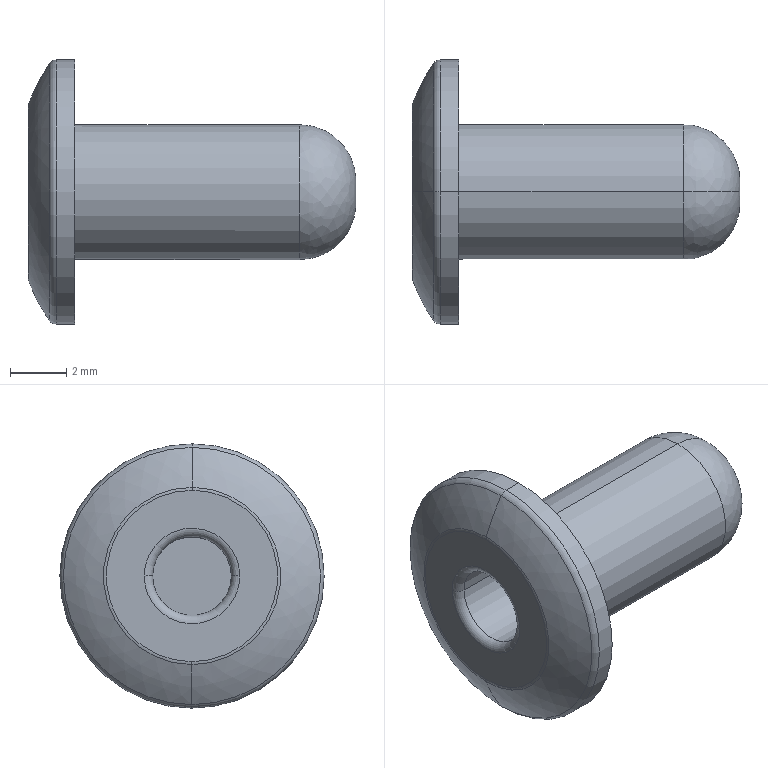Part | SolidWorks | features BaseBody 1 | 1 solid | 22 faces | box 11.653 x 9.4 x 9.401 mm | volume 238.079 mm3 | torus 8 | cylinder 6 | spline 4 | plane 4 | commonest cylinder face diameters 2.8 x2 4.8 x2 9.4 x2
STEP:
#1=CARTESIAN_POINT('',(-249.559,-95.819,-153.081));
#2=VERTEX_POINT('',#1);
#3=CARTESIAN_POINT('',(-249.804,-95.819,-153.208));
#4=VERTEX_POINT('',#3);
#5=CARTESIAN_POINT('',(-249.559,-95.819,-153.381));
#6=DIRECTION('',(0.00003827,-1.,-0.0004455));
#7=DIRECTION('',(0.0008339,-0.0004454,1.));
#8=AXIS2_PLACEMENT_3D('',#5,#6,#7);
#9=CIRCLE('',#8,0.3);
#10=EDGE_CURVE('',#2,#4,#9,.T.);
#11=ORIENTED_EDGE('',*,*,#10,.T.);
#12=CARTESIAN_POINT('',(-249.812,-95.815,-162.354));
#13=VERTEX_POINT('',#12);
#14=CARTESIAN_POINT('',(-249.808,-95.817,-157.781));
#15=DIRECTION('',(1.,0.00003864,-0.0008339));
#16=DIRECTION('',(0.0008339,-0.0004544,1.));
#17=AXIS2_PLACEMENT_3D('',#14,#15,#16);
#18=CIRCLE('',#17,4.573);
#19=EDGE_CURVE('',#4,#13,#18,.T.);
#20=ORIENTED_EDGE('',*,*,#19,.T.);
#21=CARTESIAN_POINT('',(-249.566,-95.815,-162.481));
#22=VERTEX_POINT('',#21);
#23=CARTESIAN_POINT('',(-249.566,-95.815,-162.181));
#24=DIRECTION('',(-0.00003827,1.,0.0004455));
#25=DIRECTION('',(-0.0008339,0.0004454,-1.));
#26=AXIS2_PLACEMENT_3D('',#23,#24,#25);
#27=CIRCLE('',#26,0.3);
#28=EDGE_CURVE('',#22,#13,#27,.T.);
#29=ORIENTED_EDGE('',*,*,#28,.F.);
#30=CARTESIAN_POINT('',(-249.562,-95.817,-157.781));
#31=DIRECTION('',(1.,0.00003864,-0.0008339));
#32=DIRECTION('',(0.0008339,-0.0004454,1.));
#33=AXIS2_PLACEMENT_3D('',#30,#31,#32);
#34=CIRCLE('',#33,4.7);
#35=EDGE_CURVE('',#2,#22,#34,.T.);
#36=ORIENTED_EDGE('',*,*,#35,.F.);
#37=EDGE_LOOP('',(#11,#20,#29,#36));
#38=FACE_OUTER_BOUND('',#37,.T.);
#39=CARTESIAN_POINT('',(-249.562,-95.817,-157.781));
#40=DIRECTION('',(1.,0.00003864,-0.0008339));
#41=DIRECTION('',(0.0008337,0.005616,1.));
#42=AXIS2_PLACEMENT_3D('',#39,#40,#41);
#43=TOROIDAL_SURFACE('',#42,4.4,0.3);
#44=ADVANCED_FACE('',(#38),#43,.T.);
#45=CARTESIAN_POINT('',(-248.919,-95.815,-162.481));
#46=VERTEX_POINT('',#45);
#47=CARTESIAN_POINT('',(-248.912,-95.819,-153.081));
#48=VERTEX_POINT('',#47);
#49=CARTESIAN_POINT('',(-248.916,-95.817,-157.781));
#50=DIRECTION('',(-1.,-0.00003864,0.0008339));
#51=DIRECTION('',(-0.0008339,0.0004454,-1.));
#52=AXIS2_PLACEMENT_3D('',#49,#50,#51);
#53=CIRCLE('',#52,4.7);
#54=EDGE_CURVE('',#46,#48,#53,.T.);
#55=ORIENTED_EDGE('',*,*,#54,.T.);
#56=CARTESIAN_POINT('',(-249.559,-95.819,-153.081));
#57=DIRECTION('',(1.,0.00003864,-0.0008339));
#58=VECTOR('',#57,1000.);
#59=LINE('',#56,#58);
#60=EDGE_CURVE('',#2,#48,#59,.T.);
#61=ORIENTED_EDGE('',*,*,#60,.F.);
#62=ORIENTED_EDGE('',*,*,#35,.T.);
#63=CARTESIAN_POINT('',(-249.566,-95.815,-162.481));
#64=DIRECTION('',(1.,0.00003864,-0.0008339));
#65=VECTOR('',#64,1000.);
#66=LINE('',#63,#65);
#67=EDGE_CURVE('',#22,#46,#66,.T.);
#68=ORIENTED_EDGE('',*,*,#67,.T.);
#69=EDGE_LOOP('',(#55,#61,#62,#68));
#70=FACE_OUTER_BOUND('',#69,.T.);
#71=CARTESIAN_POINT('',(-250.566,-95.817,-157.78));
#72=DIRECTION('',(1.,0.00003864,-0.0008339));
#73=DIRECTION('',(0.0008339,-0.0004454,1.));
#74=AXIS2_PLACEMENT_3D('',#71,#72,#73);
#75=CYLINDRICAL_SURFACE('',#74,4.7);
#76=ADVANCED_FACE('',(#70),#75,.T.);
#77=CARTESIAN_POINT('',(-248.916,-95.817,-157.781));
#78=DIRECTION('',(-1.,-0.00003864,0.0008339));
#79=DIRECTION('',(0.0008339,-0.0004454,1.));
#80=AXIS2_PLACEMENT_3D('',#77,#78,#79);
#81=CIRCLE('',#80,4.7);
#82=EDGE_CURVE('',#48,#46,#81,.T.);
#83=ORIENTED_EDGE('',*,*,#82,.T.);
#84=ORIENTED_EDGE('',*,*,#67,.F.);
#85=CARTESIAN_POINT('',(-249.562,-95.817,-157.781));
#86=DIRECTION('',(1.,0.00003864,-0.0008339));
#87=DIRECTION('',(-0.0008339,0.0004454,-1.));
#88=AXIS2_PLACEMENT_3D('',#85,#86,#87);
#89=CIRCLE('',#88,4.7);
#90=EDGE_CURVE('',#22,#2,#89,.T.);
#91=ORIENTED_EDGE('',*,*,#90,.T.);
#92=ORIENTED_EDGE('',*,*,#60,.T.);
#93=EDGE_LOOP('',(#83,#84,#91,#92));
#94=FACE_OUTER_BOUND('',#93,.T.);
#95=CARTESIAN_POINT('',(-250.566,-95.817,-157.78));
#96=DIRECTION('',(1.,0.00003864,-0.0008339));
#97=DIRECTION('',(0.0008339,-0.0004454,1.));
#98=AXIS2_PLACEMENT_3D('',#95,#96,#97);
#99=CYLINDRICAL_SURFACE('',#98,4.7);
#100=ADVANCED_FACE('',(#94),#99,.T.);
#101=ORIENTED_EDGE('',*,*,#28,.T.);
#102=CARTESIAN_POINT('',(-249.808,-95.817,-157.781));
#103=DIRECTION('',(1.,0.00003864,-0.0008339));
#104=DIRECTION('',(-0.0008339,0.0004544,-1.));
#105=AXIS2_PLACEMENT_3D('',#102,#103,#104);
#106=CIRCLE('',#105,4.573);
#107=EDGE_CURVE('',#13,#4,#106,.T.);
#108=ORIENTED_EDGE('',*,*,#107,.T.);
#109=ORIENTED_EDGE('',*,*,#10,.F.);
#110=ORIENTED_EDGE('',*,*,#90,.F.);
#111=EDGE_LOOP('',(#101,#108,#109,#110));
#112=FACE_OUTER_BOUND('',#111,.T.);
#113=CARTESIAN_POINT('',(-249.562,-95.817,-157.781));
#114=DIRECTION('',(1.,0.00003864,-0.0008339));
#115=DIRECTION('',(-0.0008337,-0.005616,-1.));
#116=AXIS2_PLACEMENT_3D('',#113,#114,#115);
#117=TOROIDAL_SURFACE('',#116,4.4,0.3);
#118=ADVANCED_FACE('',(#112),#117,.T.);
#119=CARTESIAN_POINT('',(-250.545,-95.819,-154.63));
#120=VERTEX_POINT('',#119);
#121=CARTESIAN_POINT('',(-249.804,-95.819,-153.208));
#122=CARTESIAN_POINT('',(-249.907,-95.819,-153.354));
#123=CARTESIAN_POINT('',(-250.1,-95.819,-153.655));
#124=CARTESIAN_POINT('',(-250.348,-95.819,-154.131));
#125=CARTESIAN_POINT('',(-250.484,-95.819,-154.462));
#126=CARTESIAN_POINT('',(-250.545,-95.819,-154.63));
#127=B_SPLINE_CURVE_WITH_KNOTS('',3,(#121,#122,#123,#124,#125,#126),.UNSPECIFIED.,.F.,.F.,(4,1,1,4),(0.,0.3333,0.6667,1.),.UNSPECIFIED.);
#128=EDGE_CURVE('',#4,#120,#127,.T.);
#129=ORIENTED_EDGE('',*,*,#128,.F.);
#130=ORIENTED_EDGE('',*,*,#107,.F.);
#131=CARTESIAN_POINT('',(-250.55,-95.816,-160.93));
#132=VERTEX_POINT('',#131);
#133=CARTESIAN_POINT('',(-249.812,-95.815,-162.354));
#134=CARTESIAN_POINT('',(-249.914,-95.815,-162.207));
#135=CARTESIAN_POINT('',(-250.107,-95.815,-161.906));
#136=CARTESIAN_POINT('',(-250.354,-95.816,-161.43));
#137=CARTESIAN_POINT('',(-250.49,-95.816,-161.098));
#138=CARTESIAN_POINT('',(-250.55,-95.816,-160.93));
#139=B_SPLINE_CURVE_WITH_KNOTS('',3,(#133,#134,#135,#136,#137,#138),.UNSPECIFIED.,.F.,.F.,(4,1,1,4),(0.000001256,0.3333,0.6667,1.),.UNSPECIFIED.);
#140=EDGE_CURVE('',#13,#132,#139,.T.);
#141=ORIENTED_EDGE('',*,*,#140,.T.);
#142=CARTESIAN_POINT('',(-250.55,-95.785,-160.93));
#143=VERTEX_POINT('',#142);
#144=CARTESIAN_POINT('',(-250.548,-95.817,-157.78));
#145=DIRECTION('',(-1.,-0.00003864,0.0008339));
#146=DIRECTION('',(-0.0008343,0.01044,-0.9999));
#147=AXIS2_PLACEMENT_3D('',#144,#145,#146);
#148=CIRCLE('',#147,3.15);
#149=EDGE_CURVE('',#143,#132,#148,.T.);
#150=ORIENTED_EDGE('',*,*,#149,.F.);
#151=CARTESIAN_POINT('',(-250.548,-95.817,-157.78));
#152=DIRECTION('',(-1.,-0.00003864,0.0008339));
#153=DIRECTION('',(-0.0008343,0.01044,-0.9999));
#154=AXIS2_PLACEMENT_3D('',#151,#152,#153);
#155=CIRCLE('',#154,3.15);
#156=EDGE_CURVE('',#120,#143,#155,.T.);
#157=ORIENTED_EDGE('',*,*,#156,.F.);
#158=EDGE_LOOP('',(#129,#130,#141,#150,#157));
#159=FACE_OUTER_BOUND('',#158,.T.);
#160=CARTESIAN_POINT('',(-250.59,-96.007,-160.811));
#161=CARTESIAN_POINT('',(-250.392,-96.043,-161.396));
#162=CARTESIAN_POINT('',(-250.107,-96.077,-161.944));
#163=CARTESIAN_POINT('',(-249.741,-96.109,-162.442));
#164=CARTESIAN_POINT('',(-250.59,-94.142,-160.927));
#165=CARTESIAN_POINT('',(-250.393,-93.818,-161.535));
#166=CARTESIAN_POINT('',(-250.108,-93.515,-162.104));
#167=CARTESIAN_POINT('',(-249.742,-93.24,-162.621));
#168=CARTESIAN_POINT('',(-250.589,-92.78,-159.647));
#169=CARTESIAN_POINT('',(-250.391,-92.194,-160.008));
#170=CARTESIAN_POINT('',(-250.106,-91.645,-160.346));
#171=CARTESIAN_POINT('',(-249.74,-91.146,-160.653));
#172=CARTESIAN_POINT('',(-250.587,-92.781,-157.779));
#173=CARTESIAN_POINT('',(-250.39,-92.195,-157.779));
#174=CARTESIAN_POINT('',(-250.104,-91.646,-157.779));
#175=CARTESIAN_POINT('',(-249.738,-91.147,-157.779));
#176=CARTESIAN_POINT('',(-250.586,-92.782,-155.91));
#177=CARTESIAN_POINT('',(-250.388,-92.196,-155.549));
#178=CARTESIAN_POINT('',(-250.102,-91.647,-155.211));
#179=CARTESIAN_POINT('',(-249.735,-91.148,-154.905));
#180=CARTESIAN_POINT('',(-250.585,-94.144,-154.631));
#181=CARTESIAN_POINT('',(-250.386,-93.822,-154.024));
#182=CARTESIAN_POINT('',(-250.1,-93.519,-153.455));
#183=CARTESIAN_POINT('',(-249.734,-93.244,-152.938));
#184=CARTESIAN_POINT('',(-250.585,-96.009,-154.75));
#185=CARTESIAN_POINT('',(-250.386,-96.047,-154.165));
#186=CARTESIAN_POINT('',(-250.1,-96.081,-153.617));
#187=CARTESIAN_POINT('',(-249.734,-96.113,-153.12));
#188=(BOUNDED_SURFACE()B_SPLINE_SURFACE(3,3,((#160,#161,#162,#163),(#164,#165,#166,#167),(#168,#169,#170,#171),(#172,#173,#174,#175),(#176,#177,#178,#179),(#180,#181,#182,#183),(#184,#185,#186,#187)),.UNSPECIFIED.,.F.,.F.,.F.)B_SPLINE_SURFACE_WITH_KNOTS((4,3,4),(4,4),(0.,1.,2.),(0.,1.),.UNSPECIFIED.)GEOMETRIC_REPRESENTATION_ITEM()RATIONAL_B_SPLINE_SURFACE(((1.194,1.185,1.185,1.194),(0.9432,0.9357,0.9357,0.9432),(0.9432,0.9357,0.9357,0.9432),(1.194,1.185,1.185,1.194),(0.9432,0.9357,0.9357,0.9432),(0.9432,0.9357,0.9357,0.9432),(1.194,1.185,1.185,1.194)))REPRESENTATION_ITEM('')SURFACE());
#189=ADVANCED_FACE('',(#159),#188,.T.);
#190=CARTESIAN_POINT('',(-250.568,-95.786,-160.829));
#191=VERTEX_POINT('',#190);
#192=CARTESIAN_POINT('',(-250.268,-95.786,-160.829));
#193=DIRECTION('',(0.00002993,-0.9999,-0.01044));
#194=DIRECTION('',(0.,0.01044,-0.9999));
#195=AXIS2_PLACEMENT_3D('',#192,#193,#194);
#196=CIRCLE('',#195,0.3);
#197=EDGE_CURVE('',#191,#143,#196,.T.);
#198=ORIENTED_EDGE('',*,*,#197,.F.);
#199=CARTESIAN_POINT('',(-250.563,-95.824,-154.732));
#200=VERTEX_POINT('',#199);
#201=CARTESIAN_POINT('',(-250.566,-95.817,-157.78));
#202=DIRECTION('',(1.,0.00003864,-0.0008339));
#203=DIRECTION('',(-0.0008343,0.01044,-0.9999));
#204=AXIS2_PLACEMENT_3D('',#201,#202,#203);
#205=CIRCLE('',#204,3.048);
#206=EDGE_CURVE('',#191,#200,#205,.T.);
#207=ORIENTED_EDGE('',*,*,#206,.T.);
#208=CARTESIAN_POINT('',(-250.263,-95.819,-154.732));
#209=DIRECTION('',(-0.00003827,1.,0.0004455));
#210=DIRECTION('',(-1.,-0.00003942,0.002586));
#211=AXIS2_PLACEMENT_3D('',#208,#209,#210);
#212=CIRCLE('',#211,0.3);
#213=EDGE_CURVE('',#200,#120,#212,.T.);
#214=ORIENTED_EDGE('',*,*,#213,.T.);
#215=ORIENTED_EDGE('',*,*,#156,.T.);
#216=EDGE_LOOP('',(#198,#207,#214,#215));
#217=FACE_OUTER_BOUND('',#216,.T.);
#218=CARTESIAN_POINT('',(-250.266,-95.817,-157.78));
#219=DIRECTION('',(1.,0.00003864,-0.0008339));
#220=DIRECTION('',(0.0008343,-0.01044,0.9999));
#221=AXIS2_PLACEMENT_3D('',#218,#219,#220);
#222=TOROIDAL_SURFACE('',#221,3.048,0.3);
#223=ADVANCED_FACE('',(#217),#222,.T.);
#224=CARTESIAN_POINT('',(-250.566,-94.116,-157.782));
#225=VERTEX_POINT('',#224);
#226=CARTESIAN_POINT('',(-250.565,-97.519,-157.734));
#227=VERTEX_POINT('',#226);
#228=CARTESIAN_POINT('',(-250.566,-94.116,-157.782));
#229=CARTESIAN_POINT('',(-250.565,-94.115,-157.554));
#230=CARTESIAN_POINT('',(-250.565,-94.153,-157.352));
#231=CARTESIAN_POINT('',(-250.565,-94.318,-156.953));
#232=CARTESIAN_POINT('',(-250.565,-94.446,-156.757));
#233=CARTESIAN_POINT('',(-250.565,-94.684,-156.509));
#234=CARTESIAN_POINT('',(-250.564,-94.813,-156.399));
#235=CARTESIAN_POINT('',(-250.564,-94.957,-156.312));
#236=CARTESIAN_POINT('',(-250.564,-95.055,-156.258));
#237=CARTESIAN_POINT('',(-250.564,-95.108,-156.233));
#238=CARTESIAN_POINT('',(-250.564,-95.261,-156.169));
#239=CARTESIAN_POINT('',(-250.564,-95.366,-156.137));
#240=CARTESIAN_POINT('',(-250.564,-95.581,-156.093));
#241=CARTESIAN_POINT('',(-250.564,-95.693,-156.082));
#242=CARTESIAN_POINT('',(-250.564,-96.028,-156.079));
#243=CARTESIAN_POINT('',(-250.564,-96.242,-156.119));
#244=CARTESIAN_POINT('',(-250.564,-96.554,-156.244));
#245=CARTESIAN_POINT('',(-250.564,-96.701,-156.32));
#246=CARTESIAN_POINT('',(-250.564,-96.834,-156.417));
#247=CARTESIAN_POINT('',(-250.564,-96.921,-156.486));
#248=CARTESIAN_POINT('',(-250.564,-96.963,-156.524));
#249=CARTESIAN_POINT('',(-250.565,-97.042,-156.601));
#250=CARTESIAN_POINT('',(-250.565,-97.079,-156.641));
#251=CARTESIAN_POINT('',(-250.565,-97.15,-156.726));
#252=CARTESIAN_POINT('',(-250.565,-97.185,-156.771));
#253=CARTESIAN_POINT('',(-250.565,-97.248,-156.861));
#254=CARTESIAN_POINT('',(-250.565,-97.276,-156.907));
#255=CARTESIAN_POINT('',(-250.565,-97.33,-157.001));
#256=CARTESIAN_POINT('',(-250.565,-97.354,-157.051));
#257=CARTESIAN_POINT('',(-250.565,-97.461,-157.291));
#258=CARTESIAN_POINT('',(-250.565,-97.508,-157.503));
#259=CARTESIAN_POINT('',(-250.565,-97.519,-157.734));
#260=B_SPLINE_CURVE_WITH_KNOTS('',3,(#228,#229,#230,#231,#232,#233,#234,#235,#236,#237,#238,#239,#240,#241,#242,#243,#244,#245,#246,#247,#248,#249,#250,#251,#252,#253,#254,#255,#256,#257,#258,#259),.UNSPECIFIED.,.F.,.F.,(4,2,2,1,2,2,2,2,2,1,2,2,2,2,2,2,4),(0.,0.125,0.25,0.3125,0.3437,0.375,0.4375,0.5,0.625,0.6875,0.7187,0.75,0.7812,0.8125,0.8437,0.875,1.),.UNSPECIFIED.);
#261=EDGE_CURVE('',#225,#227,#260,.T.);
#262=ORIENTED_EDGE('',*,*,#261,.T.);
#263=CARTESIAN_POINT('',(-250.565,-97.519,-157.778));
#264=VERTEX_POINT('',#263);
#265=CARTESIAN_POINT('',(-250.565,-97.519,-157.734));
#266=CARTESIAN_POINT('',(-250.565,-97.519,-157.738));
#267=CARTESIAN_POINT('',(-250.565,-97.519,-157.748));
#268=CARTESIAN_POINT('',(-250.565,-97.519,-157.758));
#269=CARTESIAN_POINT('',(-250.565,-97.519,-157.774));
#270=CARTESIAN_POINT('',(-250.565,-97.519,-157.778));
#271=B_SPLINE_CURVE_WITH_KNOTS('',3,(#265,#266,#267,#268,#269,#270),.UNSPECIFIED.,.F.,.F.,(4,1,1,4),(0.,0.3333,0.6667,1.),.UNSPECIFIED.);
#272=EDGE_CURVE('',#227,#264,#271,.T.);
#273=ORIENTED_EDGE('',*,*,#272,.T.);
#274=CARTESIAN_POINT('',(-250.566,-94.116,-157.826));
#275=VERTEX_POINT('',#274);
#276=CARTESIAN_POINT('',(-250.565,-97.519,-157.778));
#277=CARTESIAN_POINT('',(-250.566,-97.519,-158.006));
#278=CARTESIAN_POINT('',(-250.566,-97.482,-158.209));
#279=CARTESIAN_POINT('',(-250.566,-97.317,-158.608));
#280=CARTESIAN_POINT('',(-250.566,-97.189,-158.804));
#281=CARTESIAN_POINT('',(-250.567,-96.95,-159.051));
#282=CARTESIAN_POINT('',(-250.567,-96.822,-159.161));
#283=CARTESIAN_POINT('',(-250.567,-96.678,-159.248));
#284=CARTESIAN_POINT('',(-250.567,-96.579,-159.302));
#285=CARTESIAN_POINT('',(-250.567,-96.527,-159.327));
#286=CARTESIAN_POINT('',(-250.567,-96.374,-159.391));
#287=CARTESIAN_POINT('',(-250.567,-96.269,-159.423));
#288=CARTESIAN_POINT('',(-250.567,-96.053,-159.467));
#289=CARTESIAN_POINT('',(-250.567,-95.942,-159.478));
#290=CARTESIAN_POINT('',(-250.567,-95.607,-159.481));
#291=CARTESIAN_POINT('',(-250.567,-95.393,-159.441));
#292=CARTESIAN_POINT('',(-250.567,-95.081,-159.317));
#293=CARTESIAN_POINT('',(-250.567,-94.934,-159.241));
#294=CARTESIAN_POINT('',(-250.567,-94.8,-159.143));
#295=CARTESIAN_POINT('',(-250.567,-94.714,-159.074));
#296=CARTESIAN_POINT('',(-250.567,-94.672,-159.036));
#297=CARTESIAN_POINT('',(-250.567,-94.593,-158.959));
#298=CARTESIAN_POINT('',(-250.567,-94.556,-158.919));
#299=CARTESIAN_POINT('',(-250.566,-94.484,-158.835));
#300=CARTESIAN_POINT('',(-250.566,-94.45,-158.789));
#301=CARTESIAN_POINT('',(-250.566,-94.387,-158.699));
#302=CARTESIAN_POINT('',(-250.566,-94.358,-158.653));
#303=CARTESIAN_POINT('',(-250.566,-94.305,-158.559));
#304=CARTESIAN_POINT('',(-250.566,-94.28,-158.509));
#305=CARTESIAN_POINT('',(-250.566,-94.174,-158.269));
#306=CARTESIAN_POINT('',(-250.566,-94.126,-158.057));
#307=CARTESIAN_POINT('',(-250.566,-94.116,-157.826));
#308=B_SPLINE_CURVE_WITH_KNOTS('',3,(#276,#277,#278,#279,#280,#281,#282,#283,#284,#285,#286,#287,#288,#289,#290,#291,#292,#293,#294,#295,#296,#297,#298,#299,#300,#301,#302,#303,#304,#305,#306,#307),.UNSPECIFIED.,.F.,.F.,(4,2,2,1,2,2,2,2,2,1,2,2,2,2,2,2,4),(0.,0.125,0.25,0.3125,0.3437,0.375,0.4375,0.5,0.625,0.6875,0.7187,0.75,0.7812,0.8125,0.8437,0.875,1.),.UNSPECIFIED.);
#309=EDGE_CURVE('',#264,#275,#308,.T.);
#310=ORIENTED_EDGE('',*,*,#309,.T.);
#311=CARTESIAN_POINT('',(-250.566,-94.116,-157.826));
#312=CARTESIAN_POINT('',(-250.566,-94.116,-157.822));
#313=CARTESIAN_POINT('',(-250.566,-94.116,-157.813));
#314=CARTESIAN_POINT('',(-250.566,-94.116,-157.803));
#315=CARTESIAN_POINT('',(-250.566,-94.116,-157.786));
#316=CARTESIAN_POINT('',(-250.566,-94.116,-157.782));
#317=B_SPLINE_CURVE_WITH_KNOTS('',3,(#311,#312,#313,#314,#315,#316),.UNSPECIFIED.,.F.,.F.,(4,1,1,4),(0.,0.3333,0.6667,1.),.UNSPECIFIED.);
#318=EDGE_CURVE('',#275,#225,#317,.T.);
#319=ORIENTED_EDGE('',*,*,#318,.T.);
#320=EDGE_LOOP('',(#262,#273,#310,#319));
#321=FACE_BOUND('',#320,.T.);
#322=CARTESIAN_POINT('',(-250.563,-95.849,-154.731));
#323=VERTEX_POINT('',#322);
#324=CARTESIAN_POINT('',(-250.568,-95.811,-160.829));
#325=VERTEX_POINT('',#324);
#326=CARTESIAN_POINT('',(-250.566,-95.817,-157.78));
#327=DIRECTION('',(1.,0.00003864,-0.0008339));
#328=DIRECTION('',(0.0008343,-0.01044,0.9999));
#329=AXIS2_PLACEMENT_3D('',#326,#327,#328);
#330=CIRCLE('',#329,3.048);
#331=EDGE_CURVE('',#323,#325,#330,.T.);
#332=ORIENTED_EDGE('',*,*,#331,.F.);
#333=CARTESIAN_POINT('',(-250.566,-95.817,-157.78));
#334=DIRECTION('',(-1.,-0.00003864,0.0008339));
#335=DIRECTION('',(0.0008343,-0.01044,0.9999));
#336=AXIS2_PLACEMENT_3D('',#333,#334,#335);
#337=CIRCLE('',#336,3.049);
#338=EDGE_CURVE('',#323,#200,#337,.T.);
#339=ORIENTED_EDGE('',*,*,#338,.T.);
#340=ORIENTED_EDGE('',*,*,#206,.F.);
#341=CARTESIAN_POINT('',(-250.566,-95.817,-157.78));
#342=DIRECTION('',(-1.,-0.00003864,0.0008339));
#343=DIRECTION('',(-0.0008343,0.01044,-0.9999));
#344=AXIS2_PLACEMENT_3D('',#341,#342,#343);
#345=CIRCLE('',#344,3.049);
#346=EDGE_CURVE('',#191,#325,#345,.T.);
#347=ORIENTED_EDGE('',*,*,#346,.T.);
#348=EDGE_LOOP('',(#332,#339,#340,#347));
#349=FACE_OUTER_BOUND('',#348,.T.);
#350=CARTESIAN_POINT('',(-250.566,-95.817,-157.78));
#351=DIRECTION('',(1.,0.00003864,-0.0008339));
#352=DIRECTION('',(0.,-0.9989,-0.04628));
#353=AXIS2_PLACEMENT_3D('',#350,#351,#352);
#354=PLANE('',#353);
#355=ADVANCED_FACE('',(#321,#349),#354,.F.);
#356=CARTESIAN_POINT('',(-250.545,-95.85,-154.63));
#357=VERTEX_POINT('',#356);
#358=CARTESIAN_POINT('',(-250.263,-95.849,-154.732));
#359=DIRECTION('',(-0.00002993,0.9999,0.01044));
#360=DIRECTION('',(0.,-0.01044,0.9999));
#361=AXIS2_PLACEMENT_3D('',#358,#359,#360);
#362=CIRCLE('',#361,0.3);
#363=EDGE_CURVE('',#323,#357,#362,.T.);
#364=ORIENTED_EDGE('',*,*,#363,.F.);
#365=ORIENTED_EDGE('',*,*,#331,.T.);
#366=CARTESIAN_POINT('',(-250.268,-95.816,-160.829));
#367=DIRECTION('',(0.00003827,-1.,-0.0004455));
#368=DIRECTION('',(-1.,-0.00003786,-0.0009178));
#369=AXIS2_PLACEMENT_3D('',#366,#367,#368);
#370=CIRCLE('',#369,0.3);
#371=EDGE_CURVE('',#325,#132,#370,.T.);
#372=ORIENTED_EDGE('',*,*,#371,.T.);
#373=CARTESIAN_POINT('',(-250.548,-95.817,-157.78));
#374=DIRECTION('',(-1.,-0.00003864,0.0008339));
#375=DIRECTION('',(-0.0008339,0.0004364,-1.));
#376=AXIS2_PLACEMENT_3D('',#373,#374,#375);
#377=CIRCLE('',#376,3.15);
#378=EDGE_CURVE('',#132,#357,#377,.T.);
#379=ORIENTED_EDGE('',*,*,#378,.T.);
#380=EDGE_LOOP('',(#364,#365,#372,#379));
#381=FACE_OUTER_BOUND('',#380,.T.);
#382=CARTESIAN_POINT('',(-250.266,-95.817,-157.78));
#383=DIRECTION('',(1.,0.00003864,-0.0008339));
#384=DIRECTION('',(-0.0008343,0.01044,-0.9999));
#385=AXIS2_PLACEMENT_3D('',#382,#383,#384);
#386=TOROIDAL_SURFACE('',#385,3.048,0.3);
#387=ADVANCED_FACE('',(#381),#386,.T.);
#388=ORIENTED_EDGE('',*,*,#140,.F.);
#389=ORIENTED_EDGE('',*,*,#19,.F.);
#390=ORIENTED_EDGE('',*,*,#128,.T.);
#391=CARTESIAN_POINT('',(-250.548,-95.817,-157.78));
#392=DIRECTION('',(-1.,-0.00003864,0.0008339));
#393=DIRECTION('',(-0.0008339,0.0004364,-1.));
#394=AXIS2_PLACEMENT_3D('',#391,#392,#393);
#395=CIRCLE('',#394,3.15);
#396=EDGE_CURVE('',#357,#120,#395,.T.);
#397=ORIENTED_EDGE('',*,*,#396,.F.);
#398=ORIENTED_EDGE('',*,*,#378,.F.);
#399=EDGE_LOOP('',(#388,#389,#390,#397,#398));
#400=FACE_OUTER_BOUND('',#399,.T.);
#401=CARTESIAN_POINT('',(-250.585,-95.628,-154.749));
#402=CARTESIAN_POINT('',(-250.386,-95.592,-154.165));
#403=CARTESIAN_POINT('',(-250.1,-95.557,-153.617));
#404=CARTESIAN_POINT('',(-249.734,-95.526,-153.12));
#405=CARTESIAN_POINT('',(-250.585,-97.493,-154.633));
#406=CARTESIAN_POINT('',(-250.386,-97.817,-154.026));
#407=CARTESIAN_POINT('',(-250.1,-98.12,-153.457));
#408=CARTESIAN_POINT('',(-249.733,-98.395,-152.941));
#409=CARTESIAN_POINT('',(-250.586,-98.855,-155.913));
#410=CARTESIAN_POINT('',(-250.387,-99.441,-155.552));
#411=CARTESIAN_POINT('',(-250.102,-99.99,-155.215));
#412=CARTESIAN_POINT('',(-249.735,-100.489,-154.909));
#413=CARTESIAN_POINT('',(-250.587,-98.854,-157.781));
#414=CARTESIAN_POINT('',(-250.389,-99.44,-157.782));
#415=CARTESIAN_POINT('',(-250.104,-99.989,-157.782));
#416=CARTESIAN_POINT('',(-249.737,-100.488,-157.783));
#417=CARTESIAN_POINT('',(-250.589,-98.853,-159.65));
#418=CARTESIAN_POINT('',(-250.391,-99.439,-160.011));
#419=CARTESIAN_POINT('',(-250.106,-99.988,-160.35));
#420=CARTESIAN_POINT('',(-249.74,-100.486,-160.657));
#421=CARTESIAN_POINT('',(-250.59,-97.49,-160.929));
#422=CARTESIAN_POINT('',(-250.393,-97.813,-161.537));
#423=CARTESIAN_POINT('',(-250.107,-98.116,-162.106));
#424=CARTESIAN_POINT('',(-249.742,-98.39,-162.623));
#425=CARTESIAN_POINT('',(-250.59,-95.625,-160.811));
#426=CARTESIAN_POINT('',(-250.392,-95.588,-161.396));
#427=CARTESIAN_POINT('',(-250.107,-95.554,-161.944));
#428=CARTESIAN_POINT('',(-249.742,-95.522,-162.442));
#429=(BOUNDED_SURFACE()B_SPLINE_SURFACE(3,3,((#401,#402,#403,#404),(#405,#406,#407,#408),(#409,#410,#411,#412),(#413,#414,#415,#416),(#417,#418,#419,#420),(#421,#422,#423,#424),(#425,#426,#427,#428)),.UNSPECIFIED.,.F.,.F.,.F.)B_SPLINE_SURFACE_WITH_KNOTS((4,3,4),(4,4),(0.,1.,2.),(0.,1.),.UNSPECIFIED.)GEOMETRIC_REPRESENTATION_ITEM()RATIONAL_B_SPLINE_SURFACE(((1.194,1.185,1.185,1.194),(0.9432,0.9357,0.9357,0.9432),(0.9432,0.9357,0.9357,0.9432),(1.194,1.185,1.185,1.194),(0.9432,0.9357,0.9357,0.9432),(0.9432,0.9357,0.9357,0.9432),(1.194,1.185,1.185,1.194)))REPRESENTATION_ITEM('')SURFACE());
#430=ADVANCED_FACE('',(#400),#429,.T.);
#431=CARTESIAN_POINT('',(-250.266,-97.217,-157.781));
#432=VERTEX_POINT('',#431);
#433=CARTESIAN_POINT('',(-250.265,-97.517,-157.781));
#434=DIRECTION('',(-0.0008339,0.0004454,-1.));
#435=DIRECTION('',(-1.,-0.006413,0.0008311));
#436=AXIS2_PLACEMENT_3D('',#433,#434,#435);
#437=CIRCLE('',#436,0.3);
#438=EDGE_CURVE('',#264,#432,#437,.T.);
#439=ORIENTED_EDGE('',*,*,#438,.T.);
#440=CARTESIAN_POINT('',(-250.266,-94.417,-157.78));
#441=VERTEX_POINT('',#440);
#442=CARTESIAN_POINT('',(-250.266,-95.817,-157.78));
#443=DIRECTION('',(-1.,-0.00003864,0.0008339));
#444=DIRECTION('',(-0.00006125,0.9996,-0.02713));
#445=AXIS2_PLACEMENT_3D('',#442,#443,#444);
#446=CIRCLE('',#445,1.4);
#447=EDGE_CURVE('',#441,#432,#446,.T.);
#448=ORIENTED_EDGE('',*,*,#447,.F.);
#449=CARTESIAN_POINT('',(-250.266,-94.117,-157.78));
#450=DIRECTION('',(0.0008339,-0.0004454,1.));
#451=DIRECTION('',(-1.,0.006335,0.0008367));
#452=AXIS2_PLACEMENT_3D('',#449,#450,#451);
#453=CIRCLE('',#452,0.3);
#454=EDGE_CURVE('',#225,#441,#453,.T.);
#455=ORIENTED_EDGE('',*,*,#454,.F.);
#456=ORIENTED_EDGE('',*,*,#318,.F.);
#457=ORIENTED_EDGE('',*,*,#309,.F.);
#458=EDGE_LOOP('',(#439,#448,#455,#456,#457));
#459=FACE_OUTER_BOUND('',#458,.T.);
#460=CARTESIAN_POINT('',(-250.266,-95.817,-157.78));
#461=DIRECTION('',(-1.,-0.00003864,0.0008339));
#462=DIRECTION('',(0.00006125,-0.9996,0.02713));
#463=AXIS2_PLACEMENT_3D('',#460,#461,#462);
#464=TOROIDAL_SURFACE('',#463,1.7,0.3);
#465=ADVANCED_FACE('',(#459),#464,.T.);
#466=ORIENTED_EDGE('',*,*,#454,.T.);
#467=CARTESIAN_POINT('',(-250.266,-95.817,-157.78));
#468=DIRECTION('',(-1.,-0.00003864,0.0008339));
#469=DIRECTION('',(0.00006125,-0.9996,0.02713));
#470=AXIS2_PLACEMENT_3D('',#467,#468,#469);
#471=CIRCLE('',#470,1.4);
#472=EDGE_CURVE('',#432,#441,#471,.T.);
#473=ORIENTED_EDGE('',*,*,#472,.F.);
#474=ORIENTED_EDGE('',*,*,#438,.F.);
#475=ORIENTED_EDGE('',*,*,#272,.F.);
#476=ORIENTED_EDGE('',*,*,#261,.F.);
#477=EDGE_LOOP('',(#466,#473,#474,#475,#476));
#478=FACE_OUTER_BOUND('',#477,.T.);
#479=CARTESIAN_POINT('',(-250.266,-95.817,-157.78));
#480=DIRECTION('',(-1.,-0.00003864,0.0008339));
#481=DIRECTION('',(-0.00006125,0.9996,-0.02713));
#482=AXIS2_PLACEMENT_3D('',#479,#480,#481);
#483=TOROIDAL_SURFACE('',#482,1.7,0.3);
#484=ADVANCED_FACE('',(#478),#483,.T.);
#485=CARTESIAN_POINT('',(-245.566,-94.417,-157.784));
#486=VERTEX_POINT('',#485);
#487=CARTESIAN_POINT('',(-250.266,-94.417,-157.78));
#488=DIRECTION('',(1.,0.00003864,-0.0008339));
#489=VECTOR('',#488,1000.);
#490=LINE('',#487,#489);
#491=EDGE_CURVE('',#441,#486,#490,.T.);
#492=ORIENTED_EDGE('',*,*,#491,.T.);
#493=CARTESIAN_POINT('',(-245.566,-97.217,-157.785));
#494=VERTEX_POINT('',#493);
#495=CARTESIAN_POINT('',(-245.566,-95.817,-157.784));
#496=DIRECTION('',(1.,0.00003864,-0.0008339));
#497=DIRECTION('',(-0.00003827,1.,0.0004455));
#498=AXIS2_PLACEMENT_3D('',#495,#496,#497);
#499=CIRCLE('',#498,1.4);
#500=EDGE_CURVE('',#486,#494,#499,.T.);
#501=ORIENTED_EDGE('',*,*,#500,.T.);
#502=CARTESIAN_POINT('',(-250.266,-97.217,-157.781));
#503=DIRECTION('',(1.,0.00003864,-0.0008339));
#504=VECTOR('',#503,1000.);
#505=LINE('',#502,#504);
#506=EDGE_CURVE('',#432,#494,#505,.T.);
#507=ORIENTED_EDGE('',*,*,#506,.F.);
#508=ORIENTED_EDGE('',*,*,#472,.T.);
#509=EDGE_LOOP('',(#492,#501,#507,#508));
#510=FACE_OUTER_BOUND('',#509,.T.);
#511=CARTESIAN_POINT('',(-250.566,-95.817,-157.78));
#512=DIRECTION('',(-1.,-0.00003864,0.0008339));
#513=DIRECTION('',(-0.00003827,1.,0.0004455));
#514=AXIS2_PLACEMENT_3D('',#511,#512,#513);
#515=CYLINDRICAL_SURFACE('',#514,1.4);
#516=ADVANCED_FACE('',(#510),#515,.F.);
#517=ORIENTED_EDGE('',*,*,#506,.T.);
#518=CARTESIAN_POINT('',(-245.566,-95.817,-157.784));
#519=DIRECTION('',(1.,0.00003864,-0.0008339));
#520=DIRECTION('',(0.00003827,-1.,-0.0004455));
#521=AXIS2_PLACEMENT_3D('',#518,#519,#520);
#522=CIRCLE('',#521,1.4);
#523=EDGE_CURVE('',#494,#486,#522,.T.);
#524=ORIENTED_EDGE('',*,*,#523,.T.);
#525=ORIENTED_EDGE('',*,*,#491,.F.);
#526=ORIENTED_EDGE('',*,*,#447,.T.);
#527=EDGE_LOOP('',(#517,#524,#525,#526));
#528=FACE_OUTER_BOUND('',#527,.T.);
#529=CARTESIAN_POINT('',(-250.566,-95.817,-157.78));
#530=DIRECTION('',(-1.,-0.00003864,0.0008339));
#531=DIRECTION('',(-0.00003827,1.,0.0004455));
#532=AXIS2_PLACEMENT_3D('',#529,#530,#531);
#533=CYLINDRICAL_SURFACE('',#532,1.4);
#534=ADVANCED_FACE('',(#528),#533,.F.);
#535=ORIENTED_EDGE('',*,*,#500,.F.);
#536=ORIENTED_EDGE('',*,*,#523,.F.);
#537=EDGE_LOOP('',(#535,#536));
#538=FACE_OUTER_BOUND('',#537,.T.);
#539=CARTESIAN_POINT('',(-245.566,-95.817,-157.784));
#540=DIRECTION('',(-1.,-0.00003864,0.0008339));
#541=DIRECTION('',(-0.00003864,1.,0.));
#542=AXIS2_PLACEMENT_3D('',#539,#540,#541);
#543=PLANE('',#542);
#544=ADVANCED_FACE('',(#538),#543,.T.);
#545=CARTESIAN_POINT('',(-248.918,-95.816,-160.181));
#546=VERTEX_POINT('',#545);
#547=CARTESIAN_POINT('',(-248.914,-95.818,-155.381));
#548=VERTEX_POINT('',#547);
#549=CARTESIAN_POINT('',(-248.916,-95.817,-157.781));
#550=DIRECTION('',(1.,0.00003864,-0.0008339));
#551=DIRECTION('',(-0.0008339,0.0004454,-1.));
#552=AXIS2_PLACEMENT_3D('',#549,#550,#551);
#553=CIRCLE('',#552,2.4);
#554=EDGE_CURVE('',#546,#548,#553,.T.);
#555=ORIENTED_EDGE('',*,*,#554,.F.);
#556=CARTESIAN_POINT('',(-248.916,-95.817,-157.781));
#557=DIRECTION('',(1.,0.00003864,-0.0008339));
#558=DIRECTION('',(0.0008339,-0.0004454,1.));
#559=AXIS2_PLACEMENT_3D('',#556,#557,#558);
#560=CIRCLE('',#559,2.4);
#561=EDGE_CURVE('',#548,#546,#560,.T.);
#562=ORIENTED_EDGE('',*,*,#561,.F.);
#563=EDGE_LOOP('',(#555,#562));
#564=FACE_BOUND('',#563,.T.);
#565=ORIENTED_EDGE('',*,*,#82,.F.);
#566=ORIENTED_EDGE('',*,*,#54,.F.);
#567=EDGE_LOOP('',(#565,#566));
#568=FACE_OUTER_BOUND('',#567,.T.);
#569=CARTESIAN_POINT('',(-248.916,-95.817,-157.781));
#570=DIRECTION('',(1.,0.00003864,-0.0008339));
#571=DIRECTION('',(0.,-0.9989,-0.04628));
#572=AXIS2_PLACEMENT_3D('',#569,#570,#571);
#573=PLANE('',#572);
#574=ADVANCED_FACE('',(#564,#568),#573,.T.);
#575=CARTESIAN_POINT('',(-240.914,-95.818,-155.388));
#576=VERTEX_POINT('',#575);
#577=CARTESIAN_POINT('',(-248.914,-95.818,-155.381));
#578=DIRECTION('',(1.,0.00003796,-0.0008339));
#579=VECTOR('',#578,1000.);
#580=LINE('',#577,#579);
#581=EDGE_CURVE('',#548,#576,#580,.T.);
#582=ORIENTED_EDGE('',*,*,#581,.F.);
#583=ORIENTED_EDGE('',*,*,#561,.T.);
#584=CARTESIAN_POINT('',(-240.918,-95.816,-160.188));
#585=VERTEX_POINT('',#584);
#586=CARTESIAN_POINT('',(-248.918,-95.816,-160.181));
#587=DIRECTION('',(1.,0.00003931,-0.0008339));
#588=VECTOR('',#587,1000.);
#589=LINE('',#586,#588);
#590=EDGE_CURVE('',#546,#585,#589,.T.);
#591=ORIENTED_EDGE('',*,*,#590,.T.);
#592=CARTESIAN_POINT('',(-240.916,-95.817,-157.788));
#593=DIRECTION('',(-1.,-0.00003864,0.0008339));
#594=DIRECTION('',(-0.0008339,0.0004454,-1.));
#595=AXIS2_PLACEMENT_3D('',#592,#593,#594);
#596=CIRCLE('',#595,2.4);
#597=EDGE_CURVE('',#585,#576,#596,.T.);
#598=ORIENTED_EDGE('',*,*,#597,.T.);
#599=EDGE_LOOP('',(#582,#583,#591,#598));
#600=FACE_OUTER_BOUND('',#599,.T.);
#601=CARTESIAN_POINT('',(-248.916,-95.817,-157.781));
#602=DIRECTION('',(1.,0.00003864,-0.0008339));
#603=DIRECTION('',(0.0008339,-0.0004454,1.));
#604=AXIS2_PLACEMENT_3D('',#601,#602,#603);
#605=CYLINDRICAL_SURFACE('',#604,2.4);
#606=ADVANCED_FACE('',(#600),#605,.T.);
#607=CARTESIAN_POINT('',(-238.915,-95.817,-157.39));
#608=VERTEX_POINT('',#607);
#609=CARTESIAN_POINT('',(-240.915,-95.817,-157.388));
#610=DIRECTION('',(0.00003827,-1.,-0.0004455));
#611=DIRECTION('',(1.,0.00003864,-0.0008324));
#612=AXIS2_PLACEMENT_3D('',#609,#610,#611);
#613=CIRCLE('',#612,2.);
#614=EDGE_CURVE('',#608,#576,#613,.T.);
#615=ORIENTED_EDGE('',*,*,#614,.T.);
#616=ORIENTED_EDGE('',*,*,#597,.F.);
#617=CARTESIAN_POINT('',(-238.916,-95.817,-158.19));
#618=VERTEX_POINT('',#617);
#619=CARTESIAN_POINT('',(-240.916,-95.817,-158.188));
#620=DIRECTION('',(-0.00003827,1.,0.0004455));
#621=DIRECTION('',(1.,0.00003864,-0.0008354));
#622=AXIS2_PLACEMENT_3D('',#619,#620,#621);
#623=CIRCLE('',#622,2.);
#624=EDGE_CURVE('',#618,#585,#623,.T.);
#625=ORIENTED_EDGE('',*,*,#624,.F.);
#626=CARTESIAN_POINT('',(-238.916,-95.817,-157.79));
#627=DIRECTION('',(-1.,-0.00003864,0.0008339));
#628=DIRECTION('',(-0.0008339,0.0004454,-1.));
#629=AXIS2_PLACEMENT_3D('',#626,#627,#628);
#630=CIRCLE('',#629,0.4);
#631=EDGE_CURVE('',#618,#608,#630,.T.);
#632=ORIENTED_EDGE('',*,*,#631,.T.);
#633=EDGE_LOOP('',(#615,#616,#625,#632));
#634=FACE_OUTER_BOUND('',#633,.T.);
#635=CARTESIAN_POINT('',(-241.034,-95.11,-155.498));
#636=CARTESIAN_POINT('',(-239.75,-95.087,-155.426));
#637=CARTESIAN_POINT('',(-238.841,-95.355,-156.296));
#638=CARTESIAN_POINT('',(-238.919,-95.734,-157.522));
#639=CARTESIAN_POINT('',(-241.033,-96.795,-154.978));
#640=CARTESIAN_POINT('',(-239.749,-96.827,-154.888));
#641=CARTESIAN_POINT('',(-238.84,-96.455,-155.956));
#642=CARTESIAN_POINT('',(-238.919,-95.931,-157.461));
#643=CARTESIAN_POINT('',(-241.034,-98.214,-156.025));
#644=CARTESIAN_POINT('',(-239.75,-98.291,-155.97));
#645=CARTESIAN_POINT('',(-238.841,-97.381,-156.639));
#646=CARTESIAN_POINT('',(-238.919,-96.097,-157.584));
#647=CARTESIAN_POINT('',(-241.035,-98.213,-157.789));
#648=CARTESIAN_POINT('',(-239.751,-98.291,-157.79));
#649=CARTESIAN_POINT('',(-238.842,-97.381,-157.791));
#650=CARTESIAN_POINT('',(-238.919,-96.097,-157.79));
#651=CARTESIAN_POINT('',(-241.037,-98.213,-159.553));
#652=CARTESIAN_POINT('',(-239.753,-98.29,-159.611));
#653=CARTESIAN_POINT('',(-238.843,-97.38,-158.942));
#654=CARTESIAN_POINT('',(-238.919,-96.097,-157.996));
#655=CARTESIAN_POINT('',(-241.038,-96.793,-160.599));
#656=CARTESIAN_POINT('',(-239.754,-96.824,-160.691));
#657=CARTESIAN_POINT('',(-238.844,-96.454,-159.625));
#658=CARTESIAN_POINT('',(-238.919,-95.931,-158.118));
#659=CARTESIAN_POINT('',(-241.037,-95.108,-160.077));
#660=CARTESIAN_POINT('',(-239.754,-95.085,-160.152));
#661=CARTESIAN_POINT('',(-238.843,-95.354,-159.284));
#662=CARTESIAN_POINT('',(-238.919,-95.734,-158.057));
#663=(BOUNDED_SURFACE()B_SPLINE_SURFACE(3,3,((#635,#636,#637,#638),(#639,#640,#641,#642),(#643,#644,#645,#646),(#647,#648,#649,#650),(#651,#652,#653,#654),(#655,#656,#657,#658),(#659,#660,#661,#662)),.UNSPECIFIED.,.F.,.F.,.F.)B_SPLINE_SURFACE_WITH_KNOTS((4,3,4),(4,4),(0.,1.,2.),(0.,1.),.UNSPECIFIED.)GEOMETRIC_REPRESENTATION_ITEM()RATIONAL_B_SPLINE_SURFACE(((1.509,1.17,1.17,1.509),(1.1,0.8533,0.8533,1.1),(1.1,0.8533,0.8533,1.1),(1.509,1.17,1.17,1.509),(1.1,0.8533,0.8533,1.1),(1.1,0.8533,0.8533,1.1),(1.509,1.17,1.17,1.509)))REPRESENTATION_ITEM('')SURFACE());
#664=ADVANCED_FACE('',(#634),#663,.T.);
#665=ORIENTED_EDGE('',*,*,#631,.F.);
#666=CARTESIAN_POINT('',(-238.916,-95.817,-157.79));
#667=DIRECTION('',(-1.,-0.00003864,0.0008339));
#668=DIRECTION('',(0.0008339,-0.0004454,1.));
#669=AXIS2_PLACEMENT_3D('',#666,#667,#668);
#670=CIRCLE('',#669,0.4);
#671=EDGE_CURVE('',#608,#618,#670,.T.);
#672=ORIENTED_EDGE('',*,*,#671,.F.);
#673=EDGE_LOOP('',(#665,#672));
#674=FACE_OUTER_BOUND('',#673,.T.);
#675=CARTESIAN_POINT('',(-238.916,-95.817,-157.79));
#676=DIRECTION('',(1.,0.00003864,-0.0008339));
#677=DIRECTION('',(0.,-0.9989,-0.04628));
#678=AXIS2_PLACEMENT_3D('',#675,#676,#677);
#679=PLANE('',#678);
#680=ADVANCED_FACE('',(#674),#679,.T.);
#681=ORIENTED_EDGE('',*,*,#624,.T.);
#682=CARTESIAN_POINT('',(-240.916,-95.817,-157.788));
#683=DIRECTION('',(-1.,-0.00003864,0.0008339));
#684=DIRECTION('',(0.0008339,-0.0004454,1.));
#685=AXIS2_PLACEMENT_3D('',#682,#683,#684);
#686=CIRCLE('',#685,2.4);
#687=EDGE_CURVE('',#576,#585,#686,.T.);
#688=ORIENTED_EDGE('',*,*,#687,.F.);
#689=ORIENTED_EDGE('',*,*,#614,.F.);
#690=ORIENTED_EDGE('',*,*,#671,.T.);
#691=EDGE_LOOP('',(#681,#688,#689,#690));
#692=FACE_OUTER_BOUND('',#691,.T.);
#693=CARTESIAN_POINT('',(-241.037,-96.524,-160.078));
#694=CARTESIAN_POINT('',(-239.753,-96.547,-160.153));
#695=CARTESIAN_POINT('',(-238.843,-96.278,-159.284));
#696=CARTESIAN_POINT('',(-238.919,-95.9,-158.057));
#697=CARTESIAN_POINT('',(-241.038,-94.839,-160.598));
#698=CARTESIAN_POINT('',(-239.754,-94.807,-160.69));
#699=CARTESIAN_POINT('',(-238.844,-95.179,-159.624));
#700=CARTESIAN_POINT('',(-238.919,-95.703,-158.118));
#701=CARTESIAN_POINT('',(-241.037,-93.42,-159.551));
#702=CARTESIAN_POINT('',(-239.753,-93.343,-159.609));
#703=CARTESIAN_POINT('',(-238.843,-94.252,-158.94));
#704=CARTESIAN_POINT('',(-238.919,-95.537,-157.996));
#705=CARTESIAN_POINT('',(-241.036,-93.421,-157.787));
#706=CARTESIAN_POINT('',(-239.752,-93.343,-157.788));
#707=CARTESIAN_POINT('',(-238.842,-94.253,-157.789));
#708=CARTESIAN_POINT('',(-238.919,-95.537,-157.79));
#709=CARTESIAN_POINT('',(-241.034,-93.421,-156.023));
#710=CARTESIAN_POINT('',(-239.75,-93.344,-155.967));
#711=CARTESIAN_POINT('',(-238.841,-94.253,-156.638));
#712=CARTESIAN_POINT('',(-238.919,-95.537,-157.584));
#713=CARTESIAN_POINT('',(-241.033,-94.841,-154.977));
#714=CARTESIAN_POINT('',(-239.749,-94.81,-154.888));
#715=CARTESIAN_POINT('',(-238.841,-95.18,-155.955));
#716=CARTESIAN_POINT('',(-238.919,-95.703,-157.461));
#717=CARTESIAN_POINT('',(-241.034,-96.526,-155.499));
#718=CARTESIAN_POINT('',(-239.75,-96.549,-155.426));
#719=CARTESIAN_POINT('',(-238.841,-96.28,-156.296));
#720=CARTESIAN_POINT('',(-238.919,-95.9,-157.522));
#721=(BOUNDED_SURFACE()B_SPLINE_SURFACE(3,3,((#693,#694,#695,#696),(#697,#698,#699,#700),(#701,#702,#703,#704),(#705,#706,#707,#708),(#709,#710,#711,#712),(#713,#714,#715,#716),(#717,#718,#719,#720)),.UNSPECIFIED.,.F.,.F.,.F.)B_SPLINE_SURFACE_WITH_KNOTS((4,3,4),(4,4),(0.,1.,2.),(0.,1.),.UNSPECIFIED.)GEOMETRIC_REPRESENTATION_ITEM()RATIONAL_B_SPLINE_SURFACE(((1.509,1.17,1.17,1.509),(1.1,0.8533,0.8533,1.1),(1.1,0.8533,0.8533,1.1),(1.509,1.17,1.17,1.509),(1.1,0.8533,0.8533,1.1),(1.1,0.8533,0.8533,1.1),(1.509,1.17,1.17,1.509)))REPRESENTATION_ITEM('')SURFACE());
#722=ADVANCED_FACE('',(#692),#721,.T.);
#723=ORIENTED_EDGE('',*,*,#590,.F.);
#724=ORIENTED_EDGE('',*,*,#554,.T.);
#725=ORIENTED_EDGE('',*,*,#581,.T.);
#726=ORIENTED_EDGE('',*,*,#687,.T.);
#727=EDGE_LOOP('',(#723,#724,#725,#726));
#728=FACE_OUTER_BOUND('',#727,.T.);
#729=CARTESIAN_POINT('',(-248.916,-95.817,-157.781));
#730=DIRECTION('',(1.,0.00003864,-0.0008339));
#731=DIRECTION('',(0.0008339,-0.0004454,1.));
#732=AXIS2_PLACEMENT_3D('',#729,#730,#731);
#733=CYLINDRICAL_SURFACE('',#732,2.4);
#734=ADVANCED_FACE('',(#728),#733,.T.);
#735=ORIENTED_EDGE('',*,*,#338,.F.);
#736=ORIENTED_EDGE('',*,*,#363,.T.);
#737=ORIENTED_EDGE('',*,*,#396,.T.);
#738=ORIENTED_EDGE('',*,*,#213,.F.);
#739=EDGE_LOOP('',(#735,#736,#737,#738));
#740=FACE_OUTER_BOUND('',#739,.T.);
#741=CARTESIAN_POINT('',(-250.266,-95.817,-157.78));
#742=DIRECTION('',(1.,0.00003864,-0.0008339));
#743=DIRECTION('',(-0.0008343,0.01044,-0.9999));
#744=AXIS2_PLACEMENT_3D('',#741,#742,#743);
#745=TOROIDAL_SURFACE('',#744,3.048,0.3);
#746=ADVANCED_FACE('',(#740),#745,.T.);
#747=ORIENTED_EDGE('',*,*,#346,.F.);
#748=ORIENTED_EDGE('',*,*,#197,.T.);
#749=ORIENTED_EDGE('',*,*,#149,.T.);
#750=ORIENTED_EDGE('',*,*,#371,.F.);
#751=EDGE_LOOP('',(#747,#748,#749,#750));
#752=FACE_OUTER_BOUND('',#751,.T.);
#753=CARTESIAN_POINT('',(-250.266,-95.817,-157.78));
#754=DIRECTION('',(1.,0.00003864,-0.0008339));
#755=DIRECTION('',(0.0008343,-0.01044,0.9999));
#756=AXIS2_PLACEMENT_3D('',#753,#754,#755);
#757=TOROIDAL_SURFACE('',#756,3.048,0.3);
#758=ADVANCED_FACE('',(#752),#757,.T.);
#759=CLOSED_SHELL('',(#44,#76,#100,#118,#189,#223,#355,#387,#430,#465,#484,#516,#534,#544,#574,#606,#664,#680,#722,#734,#746,#758));
#760=MANIFOLD_SOLID_BREP('',#759);
#761=CARTESIAN_POINT('',(0.,0.,0.));
#762=DIRECTION('',(0.,0.,1.));
#763=DIRECTION('',(1.,0.,0.));
#764=AXIS2_PLACEMENT_3D('',#761,#762,#763);
#765=(LENGTH_UNIT()NAMED_UNIT(*)SI_UNIT(.MILLI.,.METRE.));
#766=UNCERTAINTY_MEASURE_WITH_UNIT(LENGTH_MEASURE(0.00001),#765,'','');
#767=(NAMED_UNIT(*)PLANE_ANGLE_UNIT()SI_UNIT($,.RADIAN.));
#768=(NAMED_UNIT(*)SI_UNIT($,.STERADIAN.)SOLID_ANGLE_UNIT());
#769=(GEOMETRIC_REPRESENTATION_CONTEXT(3)GLOBAL_UNCERTAINTY_ASSIGNED_CONTEXT((#766))GLOBAL_UNIT_ASSIGNED_CONTEXT((#765,#767,#768))REPRESENTATION_CONTEXT('',''));
#770=ADVANCED_BREP_SHAPE_REPRESENTATION('',(#760,#764),#769);